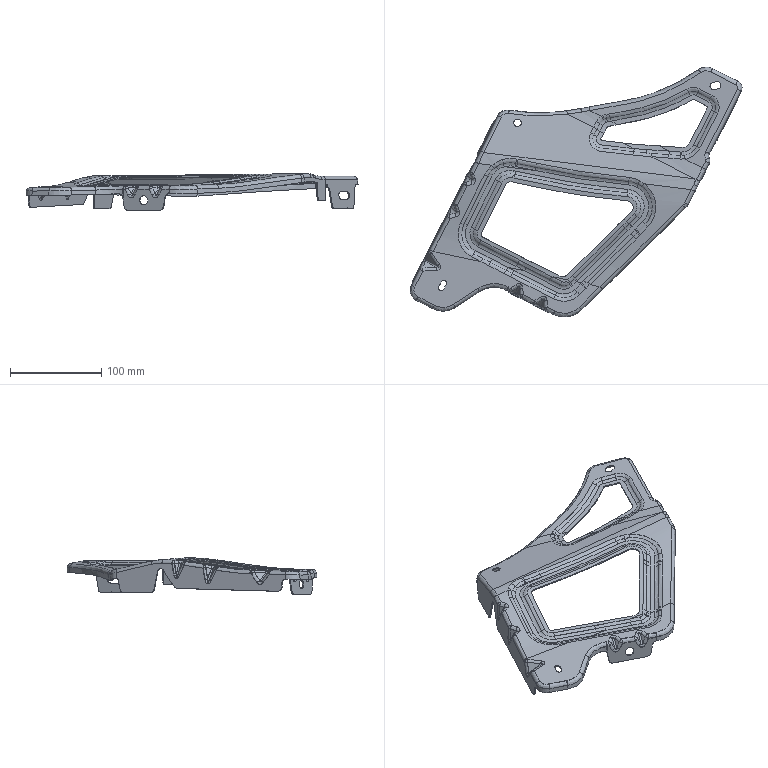Part | STEP file | 9805823280.1BPIECE_SOLIDE_FINALE_id42_x_t | 1 solid | 633 faces | box 364.658 x 274.571 x 40.313 mm | volume 68553 mm3 | spline 454 | cylinder 87 | plane 45 | other 27 | sphere 20 | commonest cylinder face diameters 5.5 x28 8 x23 3 x6 8.2 x6 4 x2 6 x2